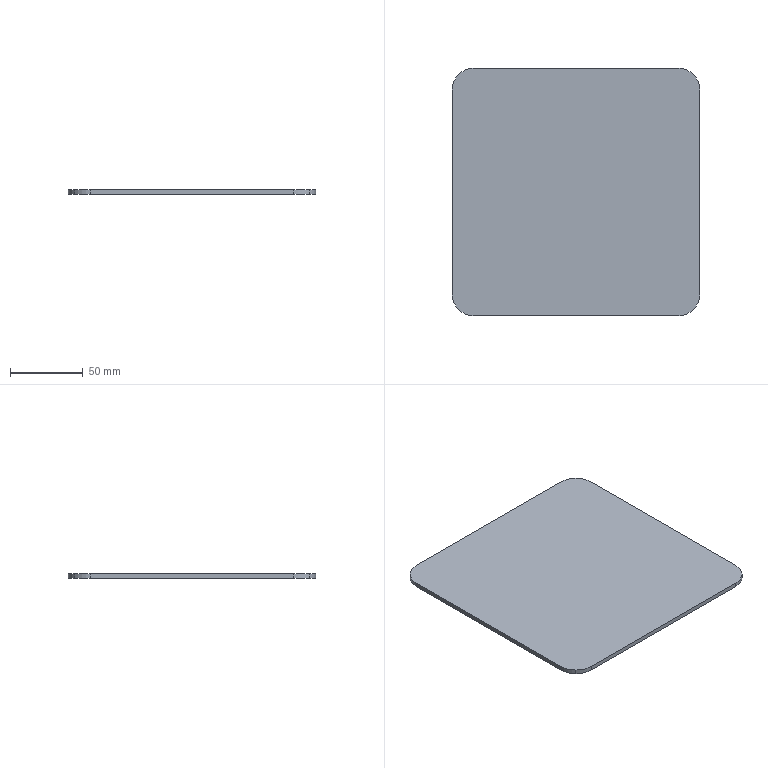Part | STEP file | Component1_2 | 1 solid | 14 faces | box 170 x 170 x 3 mm | volume 86121 mm3 | cylinder 8 | plane 6 | commonest cylinder face diameters 30 x8
STEP:
#1=CARTESIAN_POINT('',(4.393,165.607,-1.));
#2=VERTEX_POINT('',#1);
#3=CARTESIAN_POINT('',(15.,170.,-1.));
#4=VERTEX_POINT('',#3);
#5=CARTESIAN_POINT('',(15.,155.,-1.));
#6=DIRECTION('',(0.,0.,-1.));
#7=DIRECTION('',(-0.7071,0.7071,0.));
#8=AXIS2_PLACEMENT_3D('',#5,#6,#7);
#9=CIRCLE('',#8,15.);
#10=EDGE_CURVE('',#2,#4,#9,.T.);
#11=ORIENTED_EDGE('',*,*,#10,.F.);
#12=CARTESIAN_POINT('',(4.393,165.607,2.));
#13=VERTEX_POINT('',#12);
#14=CARTESIAN_POINT('',(4.393,165.607,0.));
#15=DIRECTION('',(0.,0.,1.));
#16=VECTOR('',#15,1000.);
#17=LINE('',#14,#16);
#18=EDGE_CURVE('',#2,#13,#17,.T.);
#19=ORIENTED_EDGE('',*,*,#18,.T.);
#20=CARTESIAN_POINT('',(15.,170.,2.));
#21=VERTEX_POINT('',#20);
#22=CARTESIAN_POINT('',(15.,155.,2.));
#23=DIRECTION('',(0.,0.,-1.));
#24=DIRECTION('',(-0.7071,0.7071,0.));
#25=AXIS2_PLACEMENT_3D('',#22,#23,#24);
#26=CIRCLE('',#25,15.);
#27=EDGE_CURVE('',#13,#21,#26,.T.);
#28=ORIENTED_EDGE('',*,*,#27,.T.);
#29=CARTESIAN_POINT('',(15.,170.,0.));
#30=DIRECTION('',(0.,0.,-1.));
#31=VECTOR('',#30,1000.);
#32=LINE('',#29,#31);
#33=EDGE_CURVE('',#21,#4,#32,.T.);
#34=ORIENTED_EDGE('',*,*,#33,.T.);
#35=EDGE_LOOP('',(#11,#19,#28,#34));
#36=FACE_OUTER_BOUND('',#35,.T.);
#37=CARTESIAN_POINT('',(15.,155.,0.));
#38=DIRECTION('',(0.,0.,1.));
#39=DIRECTION('',(-0.7071,0.7071,0.));
#40=AXIS2_PLACEMENT_3D('',#37,#38,#39);
#41=CYLINDRICAL_SURFACE('',#40,15.);
#42=ADVANCED_FACE('',(#36),#41,.T.);
#43=CARTESIAN_POINT('',(4.393,4.393,-1.));
#44=VERTEX_POINT('',#43);
#45=CARTESIAN_POINT('',(0.,15.,-1.));
#46=VERTEX_POINT('',#45);
#47=CARTESIAN_POINT('',(15.,15.,-1.));
#48=DIRECTION('',(0.,0.,-1.));
#49=DIRECTION('',(-0.7071,-0.7071,0.));
#50=AXIS2_PLACEMENT_3D('',#47,#48,#49);
#51=CIRCLE('',#50,15.);
#52=EDGE_CURVE('',#44,#46,#51,.T.);
#53=ORIENTED_EDGE('',*,*,#52,.F.);
#54=CARTESIAN_POINT('',(4.393,4.393,2.));
#55=VERTEX_POINT('',#54);
#56=CARTESIAN_POINT('',(4.393,4.393,0.));
#57=DIRECTION('',(0.,0.,1.));
#58=VECTOR('',#57,1000.);
#59=LINE('',#56,#58);
#60=EDGE_CURVE('',#44,#55,#59,.T.);
#61=ORIENTED_EDGE('',*,*,#60,.T.);
#62=CARTESIAN_POINT('',(0.,15.,2.));
#63=VERTEX_POINT('',#62);
#64=CARTESIAN_POINT('',(15.,15.,2.));
#65=DIRECTION('',(0.,0.,-1.));
#66=DIRECTION('',(-0.7071,-0.7071,0.));
#67=AXIS2_PLACEMENT_3D('',#64,#65,#66);
#68=CIRCLE('',#67,15.);
#69=EDGE_CURVE('',#55,#63,#68,.T.);
#70=ORIENTED_EDGE('',*,*,#69,.T.);
#71=CARTESIAN_POINT('',(0.,15.,0.));
#72=DIRECTION('',(0.,0.,-1.));
#73=VECTOR('',#72,1000.);
#74=LINE('',#71,#73);
#75=EDGE_CURVE('',#63,#46,#74,.T.);
#76=ORIENTED_EDGE('',*,*,#75,.T.);
#77=EDGE_LOOP('',(#53,#61,#70,#76));
#78=FACE_OUTER_BOUND('',#77,.T.);
#79=CARTESIAN_POINT('',(15.,15.,0.));
#80=DIRECTION('',(0.,0.,1.));
#81=DIRECTION('',(-0.7071,-0.7071,0.));
#82=AXIS2_PLACEMENT_3D('',#79,#80,#81);
#83=CYLINDRICAL_SURFACE('',#82,15.);
#84=ADVANCED_FACE('',(#78),#83,.T.);
#85=CARTESIAN_POINT('',(165.607,4.393,-1.));
#86=VERTEX_POINT('',#85);
#87=CARTESIAN_POINT('',(155.,0.,-1.));
#88=VERTEX_POINT('',#87);
#89=CARTESIAN_POINT('',(155.,15.,-1.));
#90=DIRECTION('',(0.,0.,-1.));
#91=DIRECTION('',(0.7071,-0.7071,0.));
#92=AXIS2_PLACEMENT_3D('',#89,#90,#91);
#93=CIRCLE('',#92,15.);
#94=EDGE_CURVE('',#86,#88,#93,.T.);
#95=ORIENTED_EDGE('',*,*,#94,.F.);
#96=CARTESIAN_POINT('',(165.607,4.393,2.));
#97=VERTEX_POINT('',#96);
#98=CARTESIAN_POINT('',(165.607,4.393,0.));
#99=DIRECTION('',(0.,0.,1.));
#100=VECTOR('',#99,1000.);
#101=LINE('',#98,#100);
#102=EDGE_CURVE('',#86,#97,#101,.T.);
#103=ORIENTED_EDGE('',*,*,#102,.T.);
#104=CARTESIAN_POINT('',(155.,0.,2.));
#105=VERTEX_POINT('',#104);
#106=CARTESIAN_POINT('',(155.,15.,2.));
#107=DIRECTION('',(0.,0.,-1.));
#108=DIRECTION('',(0.7071,-0.7071,0.));
#109=AXIS2_PLACEMENT_3D('',#106,#107,#108);
#110=CIRCLE('',#109,15.);
#111=EDGE_CURVE('',#97,#105,#110,.T.);
#112=ORIENTED_EDGE('',*,*,#111,.T.);
#113=CARTESIAN_POINT('',(155.,0.,0.));
#114=DIRECTION('',(0.,0.,-1.));
#115=VECTOR('',#114,1000.);
#116=LINE('',#113,#115);
#117=EDGE_CURVE('',#105,#88,#116,.T.);
#118=ORIENTED_EDGE('',*,*,#117,.T.);
#119=EDGE_LOOP('',(#95,#103,#112,#118));
#120=FACE_OUTER_BOUND('',#119,.T.);
#121=CARTESIAN_POINT('',(155.,15.,0.));
#122=DIRECTION('',(0.,0.,1.));
#123=DIRECTION('',(0.7071,-0.7071,0.));
#124=AXIS2_PLACEMENT_3D('',#121,#122,#123);
#125=CYLINDRICAL_SURFACE('',#124,15.);
#126=ADVANCED_FACE('',(#120),#125,.T.);
#127=CARTESIAN_POINT('',(165.607,165.607,-1.));
#128=VERTEX_POINT('',#127);
#129=CARTESIAN_POINT('',(170.,155.,-1.));
#130=VERTEX_POINT('',#129);
#131=CARTESIAN_POINT('',(155.,155.,-1.));
#132=DIRECTION('',(0.,0.,-1.));
#133=DIRECTION('',(0.7071,0.7071,0.));
#134=AXIS2_PLACEMENT_3D('',#131,#132,#133);
#135=CIRCLE('',#134,15.);
#136=EDGE_CURVE('',#128,#130,#135,.T.);
#137=ORIENTED_EDGE('',*,*,#136,.F.);
#138=CARTESIAN_POINT('',(165.607,165.607,2.));
#139=VERTEX_POINT('',#138);
#140=CARTESIAN_POINT('',(165.607,165.607,0.));
#141=DIRECTION('',(0.,0.,1.));
#142=VECTOR('',#141,1000.);
#143=LINE('',#140,#142);
#144=EDGE_CURVE('',#128,#139,#143,.T.);
#145=ORIENTED_EDGE('',*,*,#144,.T.);
#146=CARTESIAN_POINT('',(170.,155.,2.));
#147=VERTEX_POINT('',#146);
#148=CARTESIAN_POINT('',(155.,155.,2.));
#149=DIRECTION('',(0.,0.,-1.));
#150=DIRECTION('',(0.7071,0.7071,0.));
#151=AXIS2_PLACEMENT_3D('',#148,#149,#150);
#152=CIRCLE('',#151,15.);
#153=EDGE_CURVE('',#139,#147,#152,.T.);
#154=ORIENTED_EDGE('',*,*,#153,.T.);
#155=CARTESIAN_POINT('',(170.,155.,0.));
#156=DIRECTION('',(0.,0.,-1.));
#157=VECTOR('',#156,1000.);
#158=LINE('',#155,#157);
#159=EDGE_CURVE('',#147,#130,#158,.T.);
#160=ORIENTED_EDGE('',*,*,#159,.T.);
#161=EDGE_LOOP('',(#137,#145,#154,#160));
#162=FACE_OUTER_BOUND('',#161,.T.);
#163=CARTESIAN_POINT('',(155.,155.,0.));
#164=DIRECTION('',(0.,0.,1.));
#165=DIRECTION('',(0.7071,0.7071,0.));
#166=AXIS2_PLACEMENT_3D('',#163,#164,#165);
#167=CYLINDRICAL_SURFACE('',#166,15.);
#168=ADVANCED_FACE('',(#162),#167,.T.);
#169=CARTESIAN_POINT('',(0.,155.,2.));
#170=VERTEX_POINT('',#169);
#171=CARTESIAN_POINT('',(15.,155.,2.));
#172=DIRECTION('',(0.,0.,-1.));
#173=DIRECTION('',(-0.7071,0.7071,0.));
#174=AXIS2_PLACEMENT_3D('',#171,#172,#173);
#175=CIRCLE('',#174,15.);
#176=EDGE_CURVE('',#170,#13,#175,.T.);
#177=ORIENTED_EDGE('',*,*,#176,.F.);
#178=CARTESIAN_POINT('',(0.,170.,2.));
#179=DIRECTION('',(0.,-1.,0.));
#180=VECTOR('',#179,1000.);
#181=LINE('',#178,#180);
#182=EDGE_CURVE('',#170,#63,#181,.T.);
#183=ORIENTED_EDGE('',*,*,#182,.T.);
#184=ORIENTED_EDGE('',*,*,#69,.F.);
#185=CARTESIAN_POINT('',(15.,0.,2.));
#186=VERTEX_POINT('',#185);
#187=CARTESIAN_POINT('',(15.,15.,2.));
#188=DIRECTION('',(0.,0.,-1.));
#189=DIRECTION('',(-0.7071,-0.7071,0.));
#190=AXIS2_PLACEMENT_3D('',#187,#188,#189);
#191=CIRCLE('',#190,15.);
#192=EDGE_CURVE('',#186,#55,#191,.T.);
#193=ORIENTED_EDGE('',*,*,#192,.F.);
#194=CARTESIAN_POINT('',(0.,0.,2.));
#195=DIRECTION('',(1.,0.,0.));
#196=VECTOR('',#195,1000.);
#197=LINE('',#194,#196);
#198=EDGE_CURVE('',#186,#105,#197,.T.);
#199=ORIENTED_EDGE('',*,*,#198,.T.);
#200=ORIENTED_EDGE('',*,*,#111,.F.);
#201=CARTESIAN_POINT('',(170.,15.,2.));
#202=VERTEX_POINT('',#201);
#203=CARTESIAN_POINT('',(155.,15.,2.));
#204=DIRECTION('',(0.,0.,-1.));
#205=DIRECTION('',(0.7071,-0.7071,0.));
#206=AXIS2_PLACEMENT_3D('',#203,#204,#205);
#207=CIRCLE('',#206,15.);
#208=EDGE_CURVE('',#202,#97,#207,.T.);
#209=ORIENTED_EDGE('',*,*,#208,.F.);
#210=CARTESIAN_POINT('',(170.,0.,2.));
#211=DIRECTION('',(0.,1.,0.));
#212=VECTOR('',#211,1000.);
#213=LINE('',#210,#212);
#214=EDGE_CURVE('',#202,#147,#213,.T.);
#215=ORIENTED_EDGE('',*,*,#214,.T.);
#216=ORIENTED_EDGE('',*,*,#153,.F.);
#217=CARTESIAN_POINT('',(155.,170.,2.));
#218=VERTEX_POINT('',#217);
#219=CARTESIAN_POINT('',(155.,155.,2.));
#220=DIRECTION('',(0.,0.,-1.));
#221=DIRECTION('',(0.7071,0.7071,0.));
#222=AXIS2_PLACEMENT_3D('',#219,#220,#221);
#223=CIRCLE('',#222,15.);
#224=EDGE_CURVE('',#218,#139,#223,.T.);
#225=ORIENTED_EDGE('',*,*,#224,.F.);
#226=CARTESIAN_POINT('',(170.,170.,2.));
#227=DIRECTION('',(-1.,0.,0.));
#228=VECTOR('',#227,1000.);
#229=LINE('',#226,#228);
#230=EDGE_CURVE('',#218,#21,#229,.T.);
#231=ORIENTED_EDGE('',*,*,#230,.T.);
#232=ORIENTED_EDGE('',*,*,#27,.F.);
#233=EDGE_LOOP('',(#177,#183,#184,#193,#199,#200,#209,#215,#216,#225,#231,#232));
#234=FACE_OUTER_BOUND('',#233,.T.);
#235=CARTESIAN_POINT('',(85.,85.,2.));
#236=DIRECTION('',(0.,0.,1.));
#237=DIRECTION('',(1.,0.,0.));
#238=AXIS2_PLACEMENT_3D('',#235,#236,#237);
#239=PLANE('',#238);
#240=ADVANCED_FACE('',(#234),#239,.T.);
#241=ORIENTED_EDGE('',*,*,#33,.F.);
#242=ORIENTED_EDGE('',*,*,#230,.F.);
#243=CARTESIAN_POINT('',(155.,170.,-1.));
#244=VERTEX_POINT('',#243);
#245=CARTESIAN_POINT('',(155.,170.,0.));
#246=DIRECTION('',(0.,0.,-1.));
#247=VECTOR('',#246,1000.);
#248=LINE('',#245,#247);
#249=EDGE_CURVE('',#218,#244,#248,.T.);
#250=ORIENTED_EDGE('',*,*,#249,.T.);
#251=CARTESIAN_POINT('',(170.,170.,-1.));
#252=DIRECTION('',(1.,0.,0.));
#253=VECTOR('',#252,1000.);
#254=LINE('',#251,#253);
#255=EDGE_CURVE('',#4,#244,#254,.T.);
#256=ORIENTED_EDGE('',*,*,#255,.F.);
#257=EDGE_LOOP('',(#241,#242,#250,#256));
#258=FACE_OUTER_BOUND('',#257,.T.);
#259=CARTESIAN_POINT('',(170.,170.,0.));
#260=DIRECTION('',(0.,1.,0.));
#261=DIRECTION('',(1.,0.,0.));
#262=AXIS2_PLACEMENT_3D('',#259,#260,#261);
#263=PLANE('',#262);
#264=ADVANCED_FACE('',(#258),#263,.T.);
#265=ORIENTED_EDGE('',*,*,#144,.F.);
#266=CARTESIAN_POINT('',(155.,155.,-1.));
#267=DIRECTION('',(0.,0.,-1.));
#268=DIRECTION('',(0.7071,0.7071,0.));
#269=AXIS2_PLACEMENT_3D('',#266,#267,#268);
#270=CIRCLE('',#269,15.);
#271=EDGE_CURVE('',#244,#128,#270,.T.);
#272=ORIENTED_EDGE('',*,*,#271,.F.);
#273=ORIENTED_EDGE('',*,*,#249,.F.);
#274=ORIENTED_EDGE('',*,*,#224,.T.);
#275=EDGE_LOOP('',(#265,#272,#273,#274));
#276=FACE_OUTER_BOUND('',#275,.T.);
#277=CARTESIAN_POINT('',(155.,155.,0.));
#278=DIRECTION('',(0.,0.,1.));
#279=DIRECTION('',(0.7071,0.7071,0.));
#280=AXIS2_PLACEMENT_3D('',#277,#278,#279);
#281=CYLINDRICAL_SURFACE('',#280,15.);
#282=ADVANCED_FACE('',(#276),#281,.T.);
#283=CARTESIAN_POINT('',(170.,15.,-1.));
#284=VERTEX_POINT('',#283);
#285=CARTESIAN_POINT('',(170.,15.,0.));
#286=DIRECTION('',(0.,0.,-1.));
#287=VECTOR('',#286,1000.);
#288=LINE('',#285,#287);
#289=EDGE_CURVE('',#202,#284,#288,.T.);
#290=ORIENTED_EDGE('',*,*,#289,.T.);
#291=CARTESIAN_POINT('',(170.,0.,-1.));
#292=DIRECTION('',(0.,-1.,0.));
#293=VECTOR('',#292,1000.);
#294=LINE('',#291,#293);
#295=EDGE_CURVE('',#130,#284,#294,.T.);
#296=ORIENTED_EDGE('',*,*,#295,.F.);
#297=ORIENTED_EDGE('',*,*,#159,.F.);
#298=ORIENTED_EDGE('',*,*,#214,.F.);
#299=EDGE_LOOP('',(#290,#296,#297,#298));
#300=FACE_OUTER_BOUND('',#299,.T.);
#301=CARTESIAN_POINT('',(170.,0.,0.));
#302=DIRECTION('',(1.,0.,0.));
#303=DIRECTION('',(0.,1.,0.));
#304=AXIS2_PLACEMENT_3D('',#301,#302,#303);
#305=PLANE('',#304);
#306=ADVANCED_FACE('',(#300),#305,.T.);
#307=ORIENTED_EDGE('',*,*,#102,.F.);
#308=CARTESIAN_POINT('',(155.,15.,-1.));
#309=DIRECTION('',(0.,0.,-1.));
#310=DIRECTION('',(0.7071,-0.7071,0.));
#311=AXIS2_PLACEMENT_3D('',#308,#309,#310);
#312=CIRCLE('',#311,15.);
#313=EDGE_CURVE('',#284,#86,#312,.T.);
#314=ORIENTED_EDGE('',*,*,#313,.F.);
#315=ORIENTED_EDGE('',*,*,#289,.F.);
#316=ORIENTED_EDGE('',*,*,#208,.T.);
#317=EDGE_LOOP('',(#307,#314,#315,#316));
#318=FACE_OUTER_BOUND('',#317,.T.);
#319=CARTESIAN_POINT('',(155.,15.,0.));
#320=DIRECTION('',(0.,0.,1.));
#321=DIRECTION('',(0.7071,-0.7071,0.));
#322=AXIS2_PLACEMENT_3D('',#319,#320,#321);
#323=CYLINDRICAL_SURFACE('',#322,15.);
#324=ADVANCED_FACE('',(#318),#323,.T.);
#325=CARTESIAN_POINT('',(15.,0.,-1.));
#326=VERTEX_POINT('',#325);
#327=CARTESIAN_POINT('',(15.,0.,0.));
#328=DIRECTION('',(0.,0.,-1.));
#329=VECTOR('',#328,1000.);
#330=LINE('',#327,#329);
#331=EDGE_CURVE('',#186,#326,#330,.T.);
#332=ORIENTED_EDGE('',*,*,#331,.T.);
#333=CARTESIAN_POINT('',(0.,0.,-1.));
#334=DIRECTION('',(-1.,0.,0.));
#335=VECTOR('',#334,1000.);
#336=LINE('',#333,#335);
#337=EDGE_CURVE('',#88,#326,#336,.T.);
#338=ORIENTED_EDGE('',*,*,#337,.F.);
#339=ORIENTED_EDGE('',*,*,#117,.F.);
#340=ORIENTED_EDGE('',*,*,#198,.F.);
#341=EDGE_LOOP('',(#332,#338,#339,#340));
#342=FACE_OUTER_BOUND('',#341,.T.);
#343=CARTESIAN_POINT('',(0.,0.,0.));
#344=DIRECTION('',(0.,-1.,0.));
#345=DIRECTION('',(0.,0.,-1.));
#346=AXIS2_PLACEMENT_3D('',#343,#344,#345);
#347=PLANE('',#346);
#348=ADVANCED_FACE('',(#342),#347,.T.);
#349=ORIENTED_EDGE('',*,*,#60,.F.);
#350=CARTESIAN_POINT('',(15.,15.,-1.));
#351=DIRECTION('',(0.,0.,-1.));
#352=DIRECTION('',(-0.7071,-0.7071,0.));
#353=AXIS2_PLACEMENT_3D('',#350,#351,#352);
#354=CIRCLE('',#353,15.);
#355=EDGE_CURVE('',#326,#44,#354,.T.);
#356=ORIENTED_EDGE('',*,*,#355,.F.);
#357=ORIENTED_EDGE('',*,*,#331,.F.);
#358=ORIENTED_EDGE('',*,*,#192,.T.);
#359=EDGE_LOOP('',(#349,#356,#357,#358));
#360=FACE_OUTER_BOUND('',#359,.T.);
#361=CARTESIAN_POINT('',(15.,15.,0.));
#362=DIRECTION('',(0.,0.,1.));
#363=DIRECTION('',(-0.7071,-0.7071,0.));
#364=AXIS2_PLACEMENT_3D('',#361,#362,#363);
#365=CYLINDRICAL_SURFACE('',#364,15.);
#366=ADVANCED_FACE('',(#360),#365,.T.);
#367=CARTESIAN_POINT('',(0.,155.,-1.));
#368=VERTEX_POINT('',#367);
#369=CARTESIAN_POINT('',(0.,155.,0.));
#370=DIRECTION('',(0.,0.,-1.));
#371=VECTOR('',#370,1000.);
#372=LINE('',#369,#371);
#373=EDGE_CURVE('',#170,#368,#372,.T.);
#374=ORIENTED_EDGE('',*,*,#373,.T.);
#375=CARTESIAN_POINT('',(0.,170.,-1.));
#376=DIRECTION('',(0.,1.,0.));
#377=VECTOR('',#376,1000.);
#378=LINE('',#375,#377);
#379=EDGE_CURVE('',#46,#368,#378,.T.);
#380=ORIENTED_EDGE('',*,*,#379,.F.);
#381=ORIENTED_EDGE('',*,*,#75,.F.);
#382=ORIENTED_EDGE('',*,*,#182,.F.);
#383=EDGE_LOOP('',(#374,#380,#381,#382));
#384=FACE_OUTER_BOUND('',#383,.T.);
#385=CARTESIAN_POINT('',(0.,170.,0.));
#386=DIRECTION('',(-1.,0.,0.));
#387=DIRECTION('',(0.,0.,1.));
#388=AXIS2_PLACEMENT_3D('',#385,#386,#387);
#389=PLANE('',#388);
#390=ADVANCED_FACE('',(#384),#389,.T.);
#391=ORIENTED_EDGE('',*,*,#18,.F.);
#392=CARTESIAN_POINT('',(15.,155.,-1.));
#393=DIRECTION('',(0.,0.,-1.));
#394=DIRECTION('',(-0.7071,0.7071,0.));
#395=AXIS2_PLACEMENT_3D('',#392,#393,#394);
#396=CIRCLE('',#395,15.);
#397=EDGE_CURVE('',#368,#2,#396,.T.);
#398=ORIENTED_EDGE('',*,*,#397,.F.);
#399=ORIENTED_EDGE('',*,*,#373,.F.);
#400=ORIENTED_EDGE('',*,*,#176,.T.);
#401=EDGE_LOOP('',(#391,#398,#399,#400));
#402=FACE_OUTER_BOUND('',#401,.T.);
#403=CARTESIAN_POINT('',(15.,155.,0.));
#404=DIRECTION('',(0.,0.,1.));
#405=DIRECTION('',(-0.7071,0.7071,0.));
#406=AXIS2_PLACEMENT_3D('',#403,#404,#405);
#407=CYLINDRICAL_SURFACE('',#406,15.);
#408=ADVANCED_FACE('',(#402),#407,.T.);
#409=ORIENTED_EDGE('',*,*,#397,.T.);
#410=ORIENTED_EDGE('',*,*,#10,.T.);
#411=ORIENTED_EDGE('',*,*,#255,.T.);
#412=ORIENTED_EDGE('',*,*,#271,.T.);
#413=ORIENTED_EDGE('',*,*,#136,.T.);
#414=ORIENTED_EDGE('',*,*,#295,.T.);
#415=ORIENTED_EDGE('',*,*,#313,.T.);
#416=ORIENTED_EDGE('',*,*,#94,.T.);
#417=ORIENTED_EDGE('',*,*,#337,.T.);
#418=ORIENTED_EDGE('',*,*,#355,.T.);
#419=ORIENTED_EDGE('',*,*,#52,.T.);
#420=ORIENTED_EDGE('',*,*,#379,.T.);
#421=EDGE_LOOP('',(#409,#410,#411,#412,#413,#414,#415,#416,#417,#418,#419,#420));
#422=FACE_OUTER_BOUND('',#421,.T.);
#423=CARTESIAN_POINT('',(85.,85.,-1.));
#424=DIRECTION('',(0.,0.,1.));
#425=DIRECTION('',(1.,0.,0.));
#426=AXIS2_PLACEMENT_3D('',#423,#424,#425);
#427=PLANE('',#426);
#428=ADVANCED_FACE('',(#422),#427,.F.);
#429=CLOSED_SHELL('',(#42,#84,#126,#168,#240,#264,#282,#306,#324,#348,#366,#390,#408,#428));
#430=MANIFOLD_SOLID_BREP('',#429);
#431=CARTESIAN_POINT('',(0.,0.,0.));
#432=DIRECTION('',(0.,0.,1.));
#433=DIRECTION('',(1.,0.,0.));
#434=AXIS2_PLACEMENT_3D('',#431,#432,#433);
#435=(LENGTH_UNIT()NAMED_UNIT(*)SI_UNIT(.MILLI.,.METRE.));
#436=UNCERTAINTY_MEASURE_WITH_UNIT(LENGTH_MEASURE(0.00001),#435,'','');
#437=(NAMED_UNIT(*)PLANE_ANGLE_UNIT()SI_UNIT($,.RADIAN.));
#438=(NAMED_UNIT(*)SI_UNIT($,.STERADIAN.)SOLID_ANGLE_UNIT());
#439=(GEOMETRIC_REPRESENTATION_CONTEXT(3)GLOBAL_UNCERTAINTY_ASSIGNED_CONTEXT((#436))GLOBAL_UNIT_ASSIGNED_CONTEXT((#435,#437,#438))REPRESENTATION_CONTEXT('',''));
#440=ADVANCED_BREP_SHAPE_REPRESENTATION('',(#430,#434),#439);